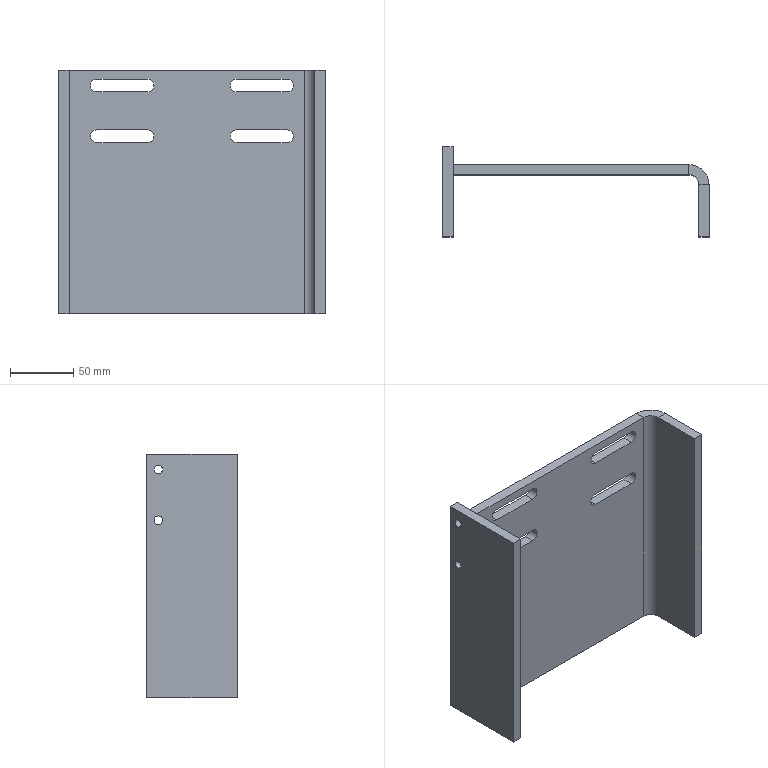Part | STEP file | 2 solids | 44 faces | box 210 x 71 x 192 mm | volume 470787 mm3 | plane 26 | cylinder 18 | commonest cylinder face diameters 10 x12 6.8 x4 16 x1 32 x1